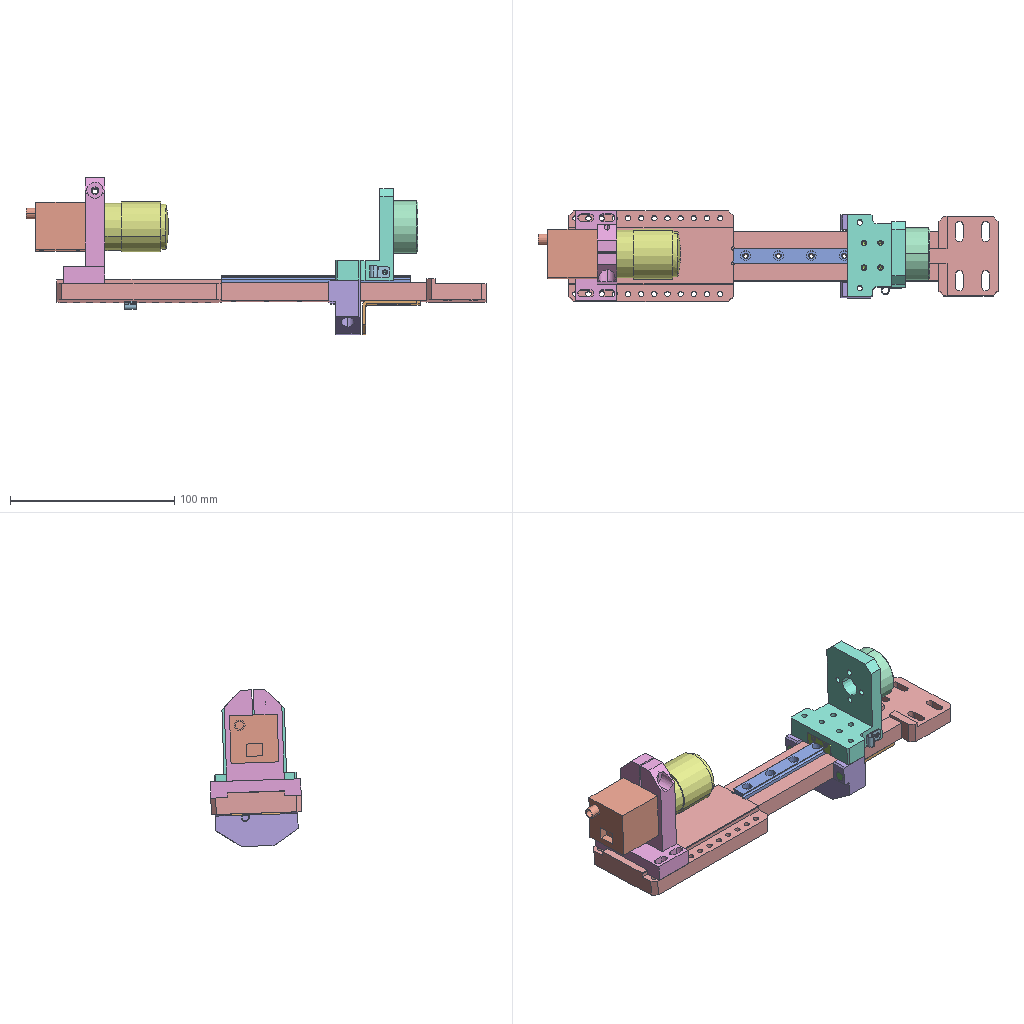Assembly | SolidWorks | 14 different items | 16 placed | box 280 x 56 x 96 mm
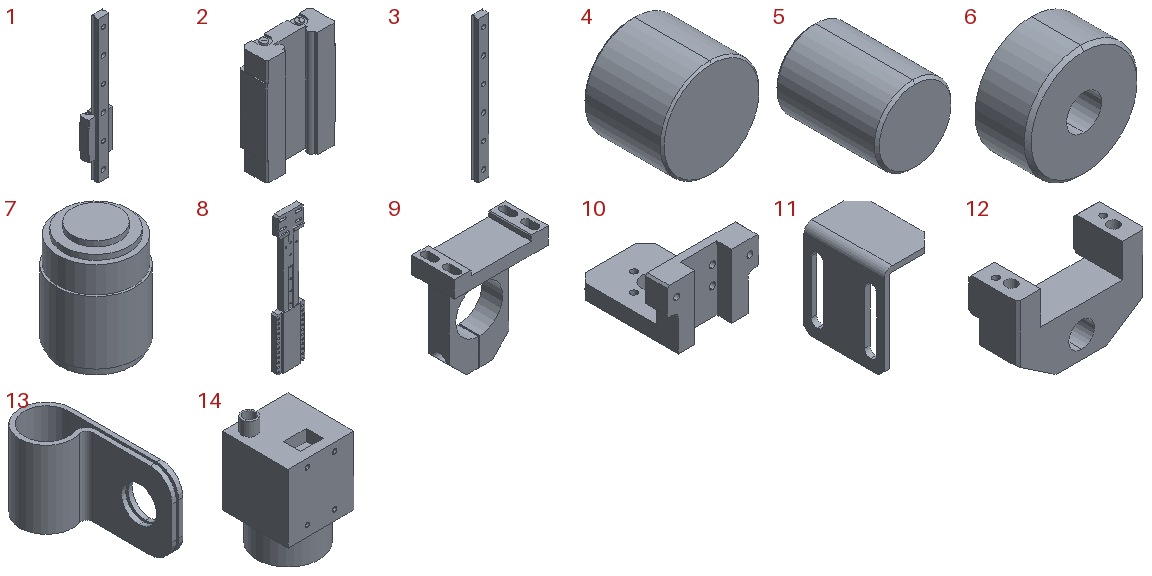Parts list (item | name | quantity | parent item | size | volume | features):
1 | (subassembly) | x1 | - | 20 x 10 x 115 mm | 8119 mm3 | -
2 | - | x1 | in 1 | 20 x 7.8 x 30 mm | 3537 mm3 | features ICE 8, RefAxis 3, 3DProfileFeature 1, Extrusion 1, LPattern 1, RevCut 1
3 | - | x1 | in 1 | 9 x 5.5 x 115 mm | 4582 mm3 | features RefAxis 6, RevCut 6, 3DProfileFeature 2, Extrusion 1
4 | - | x1 | - | 10 x 8 x 10 mm | 627.079 mm3 | features Chamfer 1, Extrusion 1
5 | - | x2 | - | 6 x 8 x 6 mm | 225.457 mm3 | features Chamfer 1, Extrusion 1
6 | - | x1 | - | 32 x 15 x 32 mm | 10684 mm3 | features 3DProfileFeature 1, Chamfer 1, CirPattern 1, Extrusion 1, HoleWzd 1
7 | - | x1 | - | 30.5 x 30.5 x 42.514 mm | 32993 mm3 | features BaseBody 2
8 | - | x1 | - | 55 x 12.8 x 261 mm | 117681 mm3 | features ICE 9, HoleWzd 4, Chamfer 3, LPattern 2, 3DProfileFeature 1, Extrusion 1, MirrorPattern 1
9 | - | x1 | - | 55 x 25 x 65 mm | 23319 mm3 | features ICE 6, Chamfer 2, Extrusion 1, HoleWzd 1
10 | - | x1 | - | 50 x 56 x 35 mm | 24108 mm3 | features ICE 6, Chamfer 2, HoleWzd 2, Extrusion 1, Fillet 1
11 | - | x1 | - | 20 x 30 x 35 mm | 2647 mm3 | features Chamfer 2, Fillet 2, ICE 2, Extrusion 1
12 | - | x1 | - | 50 x 19 x 32 mm | 14007 mm3 | features ICE 5, Chamfer 3, 3DProfileFeature 2, HoleWzd 2, Extrusion 1
13 | - | x2 | - | 4.8 x 12.4 x 7 mm | 75.143 mm3 | features Extrusion 1, Fillet 1, ICE 1
14 | - | x1 | - | - | - | features RefSurface 4, BaseBody 1, ICE 1
Mates (type | each side: item.copy, entity, surface, feature):
In the top assembly
Coincident | 8.1 face plane Boss-Extrude1 | 9.1 face plane Boss-Extrude1
DistanceDim | 9.1 face plane Boss-Extrude1 | 8.1 face plane Boss-Extrude1
Coincident | 8.1 face plane Boss-Extrude1 | 3.1 face plane Boss-Extrude1
Coincident | 2.1 face plane Boss-Extrude1 | 10.1 face plane Cut-Extrude1 | 2 times
DistanceDim | 3.1 face plane Boss-Extrude1 | 8.1 face plane Boss-Extrude1
Coincident | 8.1 face plane Boss-Extrude2 | 3.1 face plane Boss-Extrude1
Coincident | 8.1 face plane Boss-Extrude1 | 11.1 face plane Boss-Extrude1
Parallel | 8.1 face plane Boss-Extrude4 | 11.1 face plane Boss-Extrude1
Coincident | 8.1 face plane Cut-Extrude2 | 11.1 face plane Boss-Extrude1
Coincident | 10.1 face plane Boss-Extrude1 | 12.1 face plane Boss-Extrude1 | 2 times
Coincident | 10.1 face plane Boss-Extrude2 | 12.1 face plane Boss-Extrude1
Coincident | 12.1 face plane Cut-Extrude7 | 5.1 face plane Boss-Extrude1
Concentric | 12.1 face cylinder Cut-Extrude7 | 5.1 face cylinder Boss-Extrude1
Coincident | 12.1 face plane Cut-Extrude7 | 5.2 face plane Boss-Extrude1
Concentric | 12.1 face cylinder Cut-Extrude7 | 5.2 face cylinder Boss-Extrude1
DistanceDim | 11.1 face plane Boss-Extrude1 | 8.1 face plane Cut-Extrude6
Concentric | 12.1 face cylinder Cut-Extrude8 | 4.1 face cylinder Boss-Extrude1
Coincident | 12.1 face plane Cut-Extrude8 | 4.1 face plane Boss-Extrude1
Coincident | 8.1 face plane Boss-Extrude1 | 13.1 face plane Boss-Extrude1
Concentric | 8.1 face cylinder M3 Tapped Hole2 | 13.1 face cylinder Cut-Extrude1
Coincident | 10.1 face plane Cut-Extrude2 | 13.2 face plane Boss-Extrude1
Concentric | 10.1 face cylinder M3 Tapped Hole1 | 13.2 face cylinder Cut-Extrude1
Coincident | 14.1 face plane Input1 | 7.1 face plane Input1
Coincident | 9.1 face plane Boss-Extrude1 | 14.1 face plane Input1
Coincident | 6.1 face plane Boss-Extrude1 | 10.1 face plane Boss-Extrude1
Concentric | 10.1 face cylinder Boss-Extrude1 | 6.1 face cylinder Boss-Extrude1
Concentric | 2.1 face cylinder Cut-Revolve1 | 10.1 face cylinder Cut-Extrude4
Concentric | 10.1 face cylinder Cut-Extrude5 | 6.1 face cylinder CirPattern1
Concentric | 9.1 face cylinder Boss-Extrude1 | 7.1 face cylinder Input1
Concentric | 9.1 face cylinder Boss-Extrude1 | 14.1 face cylinder Boss-Extrude1
Parallel | 9.1 face plane Boss-Extrude1 | 14.1 face plane Input1
In subassembly 1
Coincident | 3.2 axis | 2.2 axis | 2 times
PlanarAngleDim | 2.2 plane | 3.2 plane